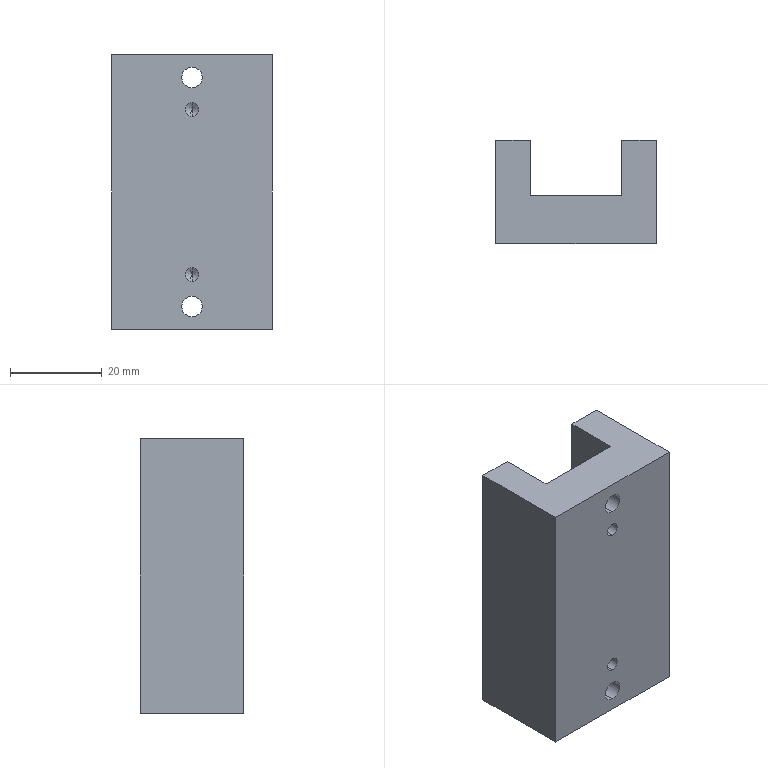Part | STEP file | PN_0034 | 1 solid | 52 faces | box 35 x 22.5 x 60 mm | volume 31897 mm3 | cylinder 24 | cone 16 | plane 12 | commonest cylinder face diameters 2.5 x12 3 x4 4.5 x4 8 x4